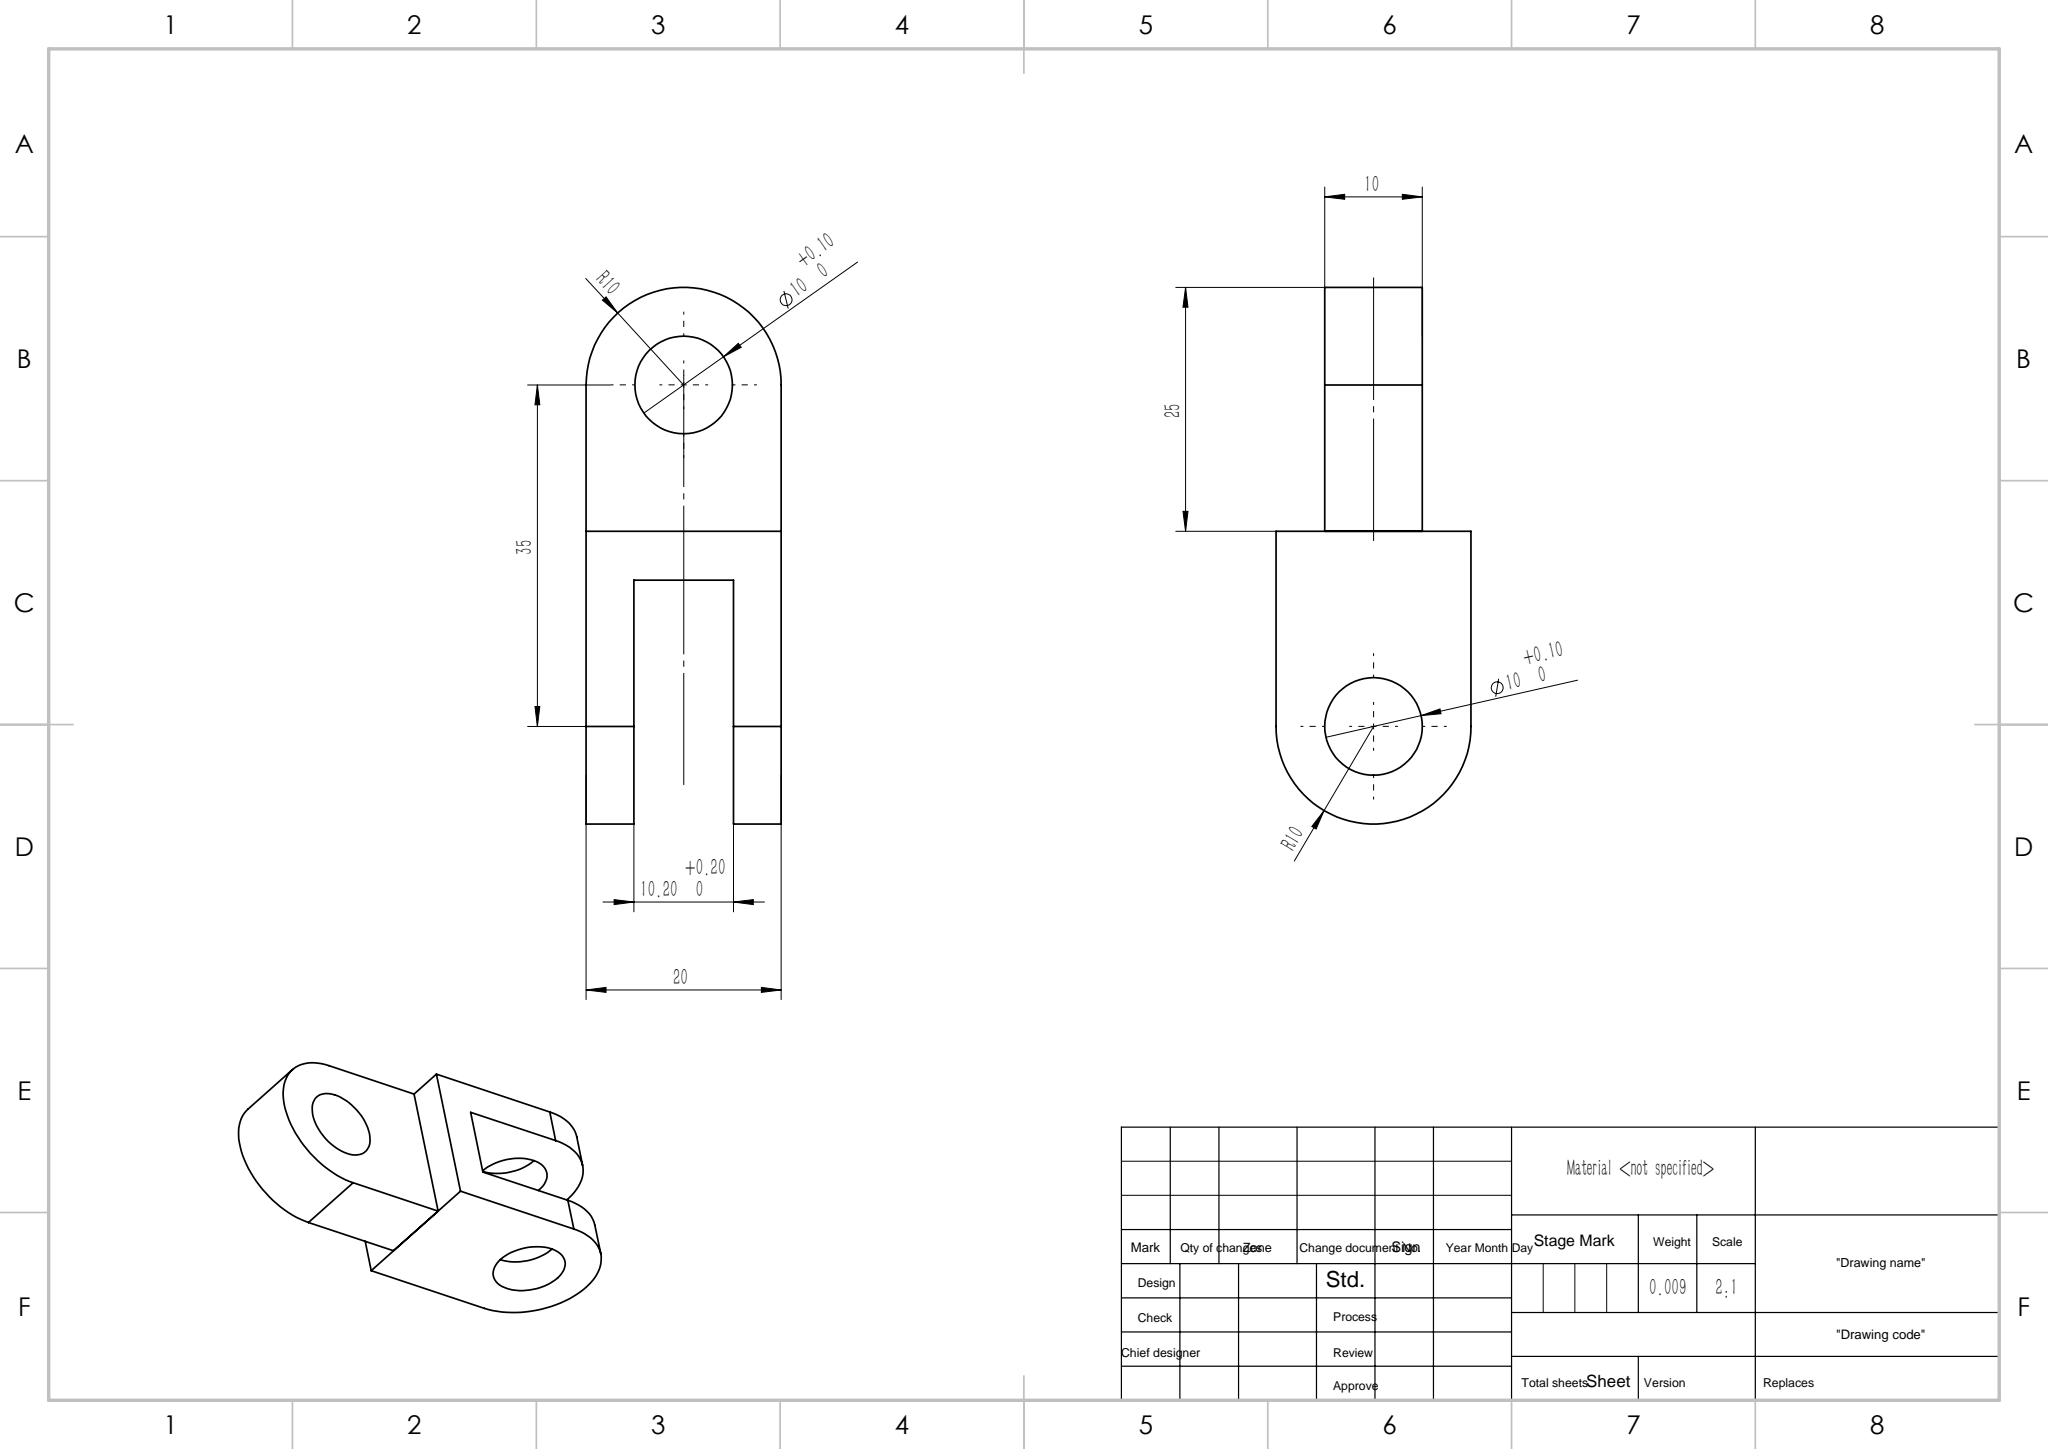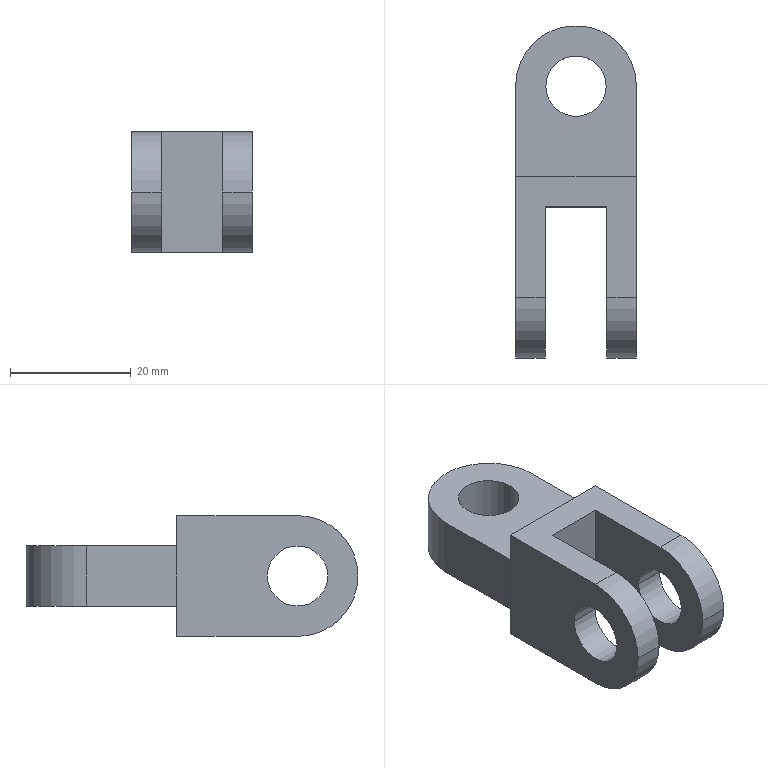Part | SolidWorks | features ICE 2, Extrusion 1 | 2 solids | 24 faces | box 20 x 55 x 20 mm | volume 9495 mm3 | plane 13 | cylinder 11 | commonest cylinder face diameters 10 x6 20 x5
STEP:
#1=CARTESIAN_POINT('',(-5.,0.,10.));
#2=VERTEX_POINT('',#1);
#3=CARTESIAN_POINT('',(5.,0.,10.));
#4=VERTEX_POINT('',#3);
#5=CARTESIAN_POINT('',(0.,0.,10.));
#6=DIRECTION('',(0.,0.,1.));
#7=DIRECTION('',(1.,0.,0.));
#8=AXIS2_PLACEMENT_3D('',#5,#6,#7);
#9=CIRCLE('',#8,5.);
#10=EDGE_CURVE('',#2,#4,#9,.T.);
#11=ORIENTED_EDGE('',*,*,#10,.T.);
#12=CARTESIAN_POINT('',(5.,0.,0.));
#13=VERTEX_POINT('',#12);
#14=CARTESIAN_POINT('',(5.,0.,10.));
#15=DIRECTION('',(0.,0.,-1.));
#16=VECTOR('',#15,1000.);
#17=LINE('',#14,#16);
#18=EDGE_CURVE('',#4,#13,#17,.T.);
#19=ORIENTED_EDGE('',*,*,#18,.T.);
#20=CARTESIAN_POINT('',(-5.,0.,0.));
#21=VERTEX_POINT('',#20);
#22=CARTESIAN_POINT('',(0.,0.,0.));
#23=DIRECTION('',(0.,0.,1.));
#24=DIRECTION('',(1.,0.,0.));
#25=AXIS2_PLACEMENT_3D('',#22,#23,#24);
#26=CIRCLE('',#25,5.);
#27=EDGE_CURVE('',#21,#13,#26,.T.);
#28=ORIENTED_EDGE('',*,*,#27,.F.);
#29=CARTESIAN_POINT('',(-5.,0.,10.));
#30=DIRECTION('',(0.,0.,-1.));
#31=VECTOR('',#30,1000.);
#32=LINE('',#29,#31);
#33=EDGE_CURVE('',#2,#21,#32,.T.);
#34=ORIENTED_EDGE('',*,*,#33,.F.);
#35=EDGE_LOOP('',(#11,#19,#28,#34));
#36=FACE_OUTER_BOUND('',#35,.T.);
#37=CARTESIAN_POINT('',(0.,0.,10.));
#38=DIRECTION('',(0.,0.,-1.));
#39=DIRECTION('',(-1.,0.,0.));
#40=AXIS2_PLACEMENT_3D('',#37,#38,#39);
#41=CYLINDRICAL_SURFACE('',#40,5.);
#42=ADVANCED_FACE('',(#36),#41,.F.);
#43=CARTESIAN_POINT('',(10.,0.,10.));
#44=VERTEX_POINT('',#43);
#45=CARTESIAN_POINT('',(-10.,0.,10.));
#46=VERTEX_POINT('',#45);
#47=CARTESIAN_POINT('',(0.,0.,10.));
#48=DIRECTION('',(0.,0.,1.));
#49=DIRECTION('',(1.,0.,0.));
#50=AXIS2_PLACEMENT_3D('',#47,#48,#49);
#51=CIRCLE('',#50,10.);
#52=EDGE_CURVE('',#44,#46,#51,.T.);
#53=ORIENTED_EDGE('',*,*,#52,.T.);
#54=CARTESIAN_POINT('',(-10.,-15.,10.));
#55=VERTEX_POINT('',#54);
#56=CARTESIAN_POINT('',(-10.,0.,10.));
#57=DIRECTION('',(0.,-1.,0.));
#58=VECTOR('',#57,1000.);
#59=LINE('',#56,#58);
#60=EDGE_CURVE('',#46,#55,#59,.T.);
#61=ORIENTED_EDGE('',*,*,#60,.T.);
#62=CARTESIAN_POINT('',(10.,-15.,10.));
#63=VERTEX_POINT('',#62);
#64=CARTESIAN_POINT('',(-10.,-15.,10.));
#65=DIRECTION('',(1.,0.,0.));
#66=VECTOR('',#65,1000.);
#67=LINE('',#64,#66);
#68=EDGE_CURVE('',#55,#63,#67,.T.);
#69=ORIENTED_EDGE('',*,*,#68,.T.);
#70=CARTESIAN_POINT('',(10.,-15.,10.));
#71=DIRECTION('',(0.,1.,0.));
#72=VECTOR('',#71,1000.);
#73=LINE('',#70,#72);
#74=EDGE_CURVE('',#63,#44,#73,.T.);
#75=ORIENTED_EDGE('',*,*,#74,.T.);
#76=EDGE_LOOP('',(#53,#61,#69,#75));
#77=FACE_OUTER_BOUND('',#76,.T.);
#78=ORIENTED_EDGE('',*,*,#10,.F.);
#79=CARTESIAN_POINT('',(0.,0.,10.));
#80=DIRECTION('',(0.,0.,1.));
#81=DIRECTION('',(1.,0.,0.));
#82=AXIS2_PLACEMENT_3D('',#79,#80,#81);
#83=CIRCLE('',#82,5.);
#84=EDGE_CURVE('',#4,#2,#83,.T.);
#85=ORIENTED_EDGE('',*,*,#84,.F.);
#86=EDGE_LOOP('',(#78,#85));
#87=FACE_BOUND('',#86,.T.);
#88=CARTESIAN_POINT('',(0.,0.,10.));
#89=DIRECTION('',(0.,0.,1.));
#90=DIRECTION('',(1.,0.,0.));
#91=AXIS2_PLACEMENT_3D('',#88,#89,#90);
#92=PLANE('',#91);
#93=ADVANCED_FACE('',(#77,#87),#92,.T.);
#94=CARTESIAN_POINT('',(10.,0.,0.));
#95=VERTEX_POINT('',#94);
#96=CARTESIAN_POINT('',(-10.,0.,0.));
#97=VERTEX_POINT('',#96);
#98=CARTESIAN_POINT('',(0.,0.,0.));
#99=DIRECTION('',(0.,0.,1.));
#100=DIRECTION('',(1.,0.,0.));
#101=AXIS2_PLACEMENT_3D('',#98,#99,#100);
#102=CIRCLE('',#101,10.);
#103=EDGE_CURVE('',#95,#97,#102,.T.);
#104=ORIENTED_EDGE('',*,*,#103,.F.);
#105=CARTESIAN_POINT('',(10.,-15.,0.));
#106=VERTEX_POINT('',#105);
#107=CARTESIAN_POINT('',(10.,-15.,0.));
#108=DIRECTION('',(0.,1.,0.));
#109=VECTOR('',#108,1000.);
#110=LINE('',#107,#109);
#111=EDGE_CURVE('',#106,#95,#110,.T.);
#112=ORIENTED_EDGE('',*,*,#111,.F.);
#113=CARTESIAN_POINT('',(-10.,-15.,0.));
#114=VERTEX_POINT('',#113);
#115=CARTESIAN_POINT('',(-10.,-15.,0.));
#116=DIRECTION('',(1.,0.,0.));
#117=VECTOR('',#116,1000.);
#118=LINE('',#115,#117);
#119=EDGE_CURVE('',#114,#106,#118,.T.);
#120=ORIENTED_EDGE('',*,*,#119,.F.);
#121=CARTESIAN_POINT('',(-10.,0.,0.));
#122=DIRECTION('',(0.,-1.,0.));
#123=VECTOR('',#122,1000.);
#124=LINE('',#121,#123);
#125=EDGE_CURVE('',#97,#114,#124,.T.);
#126=ORIENTED_EDGE('',*,*,#125,.F.);
#127=EDGE_LOOP('',(#104,#112,#120,#126));
#128=FACE_OUTER_BOUND('',#127,.T.);
#129=ORIENTED_EDGE('',*,*,#27,.T.);
#130=CARTESIAN_POINT('',(0.,0.,0.));
#131=DIRECTION('',(0.,0.,1.));
#132=DIRECTION('',(1.,0.,0.));
#133=AXIS2_PLACEMENT_3D('',#130,#131,#132);
#134=CIRCLE('',#133,5.);
#135=EDGE_CURVE('',#13,#21,#134,.T.);
#136=ORIENTED_EDGE('',*,*,#135,.T.);
#137=EDGE_LOOP('',(#129,#136));
#138=FACE_BOUND('',#137,.T.);
#139=CARTESIAN_POINT('',(0.,0.,0.));
#140=DIRECTION('',(0.,0.,1.));
#141=DIRECTION('',(1.,0.,0.));
#142=AXIS2_PLACEMENT_3D('',#139,#140,#141);
#143=PLANE('',#142);
#144=ADVANCED_FACE('',(#128,#138),#143,.F.);
#145=ORIENTED_EDGE('',*,*,#103,.T.);
#146=CARTESIAN_POINT('',(-10.,0.,10.));
#147=DIRECTION('',(0.,0.,-1.));
#148=VECTOR('',#147,1000.);
#149=LINE('',#146,#148);
#150=EDGE_CURVE('',#46,#97,#149,.T.);
#151=ORIENTED_EDGE('',*,*,#150,.F.);
#152=ORIENTED_EDGE('',*,*,#52,.F.);
#153=CARTESIAN_POINT('',(10.,0.,10.));
#154=DIRECTION('',(0.,0.,-1.));
#155=VECTOR('',#154,1000.);
#156=LINE('',#153,#155);
#157=EDGE_CURVE('',#44,#95,#156,.T.);
#158=ORIENTED_EDGE('',*,*,#157,.T.);
#159=EDGE_LOOP('',(#145,#151,#152,#158));
#160=FACE_OUTER_BOUND('',#159,.T.);
#161=CARTESIAN_POINT('',(0.,0.,10.));
#162=DIRECTION('',(0.,0.,-1.));
#163=DIRECTION('',(-1.,0.,0.));
#164=AXIS2_PLACEMENT_3D('',#161,#162,#163);
#165=CYLINDRICAL_SURFACE('',#164,10.);
#166=ADVANCED_FACE('',(#160),#165,.T.);
#167=ORIENTED_EDGE('',*,*,#125,.T.);
#168=CARTESIAN_POINT('',(-10.,-15.,10.));
#169=DIRECTION('',(0.,0.,-1.));
#170=VECTOR('',#169,1000.);
#171=LINE('',#168,#170);
#172=EDGE_CURVE('',#55,#114,#171,.T.);
#173=ORIENTED_EDGE('',*,*,#172,.F.);
#174=ORIENTED_EDGE('',*,*,#60,.F.);
#175=ORIENTED_EDGE('',*,*,#150,.T.);
#176=EDGE_LOOP('',(#167,#173,#174,#175));
#177=FACE_OUTER_BOUND('',#176,.T.);
#178=CARTESIAN_POINT('',(-10.,0.,10.));
#179=DIRECTION('',(1.,0.,0.));
#180=DIRECTION('',(0.,1.,0.));
#181=AXIS2_PLACEMENT_3D('',#178,#179,#180);
#182=PLANE('',#181);
#183=ADVANCED_FACE('',(#177),#182,.F.);
#184=ORIENTED_EDGE('',*,*,#119,.T.);
#185=CARTESIAN_POINT('',(10.,-15.,10.));
#186=DIRECTION('',(0.,0.,-1.));
#187=VECTOR('',#186,1000.);
#188=LINE('',#185,#187);
#189=EDGE_CURVE('',#63,#106,#188,.T.);
#190=ORIENTED_EDGE('',*,*,#189,.F.);
#191=ORIENTED_EDGE('',*,*,#68,.F.);
#192=ORIENTED_EDGE('',*,*,#172,.T.);
#193=EDGE_LOOP('',(#184,#190,#191,#192));
#194=FACE_OUTER_BOUND('',#193,.T.);
#195=CARTESIAN_POINT('',(-10.,-15.,10.));
#196=DIRECTION('',(0.,1.,0.));
#197=DIRECTION('',(0.,0.,1.));
#198=AXIS2_PLACEMENT_3D('',#195,#196,#197);
#199=PLANE('',#198);
#200=ADVANCED_FACE('',(#194),#199,.F.);
#201=ORIENTED_EDGE('',*,*,#111,.T.);
#202=ORIENTED_EDGE('',*,*,#157,.F.);
#203=ORIENTED_EDGE('',*,*,#74,.F.);
#204=ORIENTED_EDGE('',*,*,#189,.T.);
#205=EDGE_LOOP('',(#201,#202,#203,#204));
#206=FACE_OUTER_BOUND('',#205,.T.);
#207=CARTESIAN_POINT('',(10.,-15.,10.));
#208=DIRECTION('',(-1.,0.,0.));
#209=DIRECTION('',(0.,-1.,0.));
#210=AXIS2_PLACEMENT_3D('',#207,#208,#209);
#211=PLANE('',#210);
#212=ADVANCED_FACE('',(#206),#211,.F.);
#213=ORIENTED_EDGE('',*,*,#18,.F.);
#214=ORIENTED_EDGE('',*,*,#84,.T.);
#215=ORIENTED_EDGE('',*,*,#33,.T.);
#216=ORIENTED_EDGE('',*,*,#135,.F.);
#217=EDGE_LOOP('',(#213,#214,#215,#216));
#218=FACE_OUTER_BOUND('',#217,.T.);
#219=CARTESIAN_POINT('',(0.,0.,10.));
#220=DIRECTION('',(0.,0.,-1.));
#221=DIRECTION('',(-1.,0.,0.));
#222=AXIS2_PLACEMENT_3D('',#219,#220,#221);
#223=CYLINDRICAL_SURFACE('',#222,5.);
#224=ADVANCED_FACE('',(#218),#223,.F.);
#225=CLOSED_SHELL('',(#42,#93,#144,#166,#183,#200,#212,#224));
#226=MANIFOLD_SOLID_BREP('',#225);
#227=CARTESIAN_POINT('',(10.,-30.,5.));
#228=VERTEX_POINT('',#227);
#229=CARTESIAN_POINT('',(10.,-40.,5.));
#230=VERTEX_POINT('',#229);
#231=CARTESIAN_POINT('',(10.,-35.,5.));
#232=DIRECTION('',(-1.,0.,0.));
#233=DIRECTION('',(0.,-1.,0.));
#234=AXIS2_PLACEMENT_3D('',#231,#232,#233);
#235=CIRCLE('',#234,5.);
#236=EDGE_CURVE('',#228,#230,#235,.T.);
#237=ORIENTED_EDGE('',*,*,#236,.F.);
#238=CARTESIAN_POINT('',(5.1,-30.,5.));
#239=VERTEX_POINT('',#238);
#240=CARTESIAN_POINT('',(10.,-30.,5.));
#241=DIRECTION('',(-1.,0.,0.));
#242=VECTOR('',#241,1000.);
#243=LINE('',#240,#242);
#244=EDGE_CURVE('',#228,#239,#243,.T.);
#245=ORIENTED_EDGE('',*,*,#244,.T.);
#246=CARTESIAN_POINT('',(5.1,-40.,5.));
#247=VERTEX_POINT('',#246);
#248=CARTESIAN_POINT('',(5.1,-35.,5.));
#249=DIRECTION('',(-1.,0.,0.));
#250=DIRECTION('',(0.,1.,0.));
#251=AXIS2_PLACEMENT_3D('',#248,#249,#250);
#252=CIRCLE('',#251,5.);
#253=EDGE_CURVE('',#239,#247,#252,.T.);
#254=ORIENTED_EDGE('',*,*,#253,.T.);
#255=CARTESIAN_POINT('',(10.,-40.,5.));
#256=DIRECTION('',(-1.,0.,0.));
#257=VECTOR('',#256,1000.);
#258=LINE('',#255,#257);
#259=EDGE_CURVE('',#230,#247,#258,.T.);
#260=ORIENTED_EDGE('',*,*,#259,.F.);
#261=EDGE_LOOP('',(#237,#245,#254,#260));
#262=FACE_OUTER_BOUND('',#261,.T.);
#263=CARTESIAN_POINT('',(10.,-35.,5.));
#264=DIRECTION('',(-1.,0.,0.));
#265=DIRECTION('',(0.,-1.,0.));
#266=AXIS2_PLACEMENT_3D('',#263,#264,#265);
#267=CYLINDRICAL_SURFACE('',#266,5.);
#268=ADVANCED_FACE('',(#262),#267,.F.);
#269=CARTESIAN_POINT('',(10.,-35.,-5.));
#270=VERTEX_POINT('',#269);
#271=CARTESIAN_POINT('',(10.,-45.,5.));
#272=VERTEX_POINT('',#271);
#273=CARTESIAN_POINT('',(10.,-35.,5.));
#274=DIRECTION('',(-1.,0.,0.));
#275=DIRECTION('',(0.,-1.,0.));
#276=AXIS2_PLACEMENT_3D('',#273,#274,#275);
#277=CIRCLE('',#276,10.);
#278=EDGE_CURVE('',#270,#272,#277,.T.);
#279=ORIENTED_EDGE('',*,*,#278,.T.);
#280=CARTESIAN_POINT('',(5.1,-45.,5.));
#281=VERTEX_POINT('',#280);
#282=CARTESIAN_POINT('',(10.,-45.,5.));
#283=DIRECTION('',(-1.,0.,0.));
#284=VECTOR('',#283,1000.);
#285=LINE('',#282,#284);
#286=EDGE_CURVE('',#272,#281,#285,.T.);
#287=ORIENTED_EDGE('',*,*,#286,.T.);
#288=CARTESIAN_POINT('',(5.1,-35.,-5.));
#289=VERTEX_POINT('',#288);
#290=CARTESIAN_POINT('',(5.1,-35.,5.));
#291=DIRECTION('',(-1.,0.,0.));
#292=DIRECTION('',(0.,1.,0.));
#293=AXIS2_PLACEMENT_3D('',#290,#291,#292);
#294=CIRCLE('',#293,10.);
#295=EDGE_CURVE('',#289,#281,#294,.T.);
#296=ORIENTED_EDGE('',*,*,#295,.F.);
#297=CARTESIAN_POINT('',(10.,-35.,-5.));
#298=DIRECTION('',(-1.,0.,0.));
#299=VECTOR('',#298,1000.);
#300=LINE('',#297,#299);
#301=EDGE_CURVE('',#270,#289,#300,.T.);
#302=ORIENTED_EDGE('',*,*,#301,.F.);
#303=EDGE_LOOP('',(#279,#287,#296,#302));
#304=FACE_OUTER_BOUND('',#303,.T.);
#305=CARTESIAN_POINT('',(10.,-35.,5.));
#306=DIRECTION('',(-1.,0.,0.));
#307=DIRECTION('',(0.,-1.,0.));
#308=AXIS2_PLACEMENT_3D('',#305,#306,#307);
#309=CYLINDRICAL_SURFACE('',#308,10.);
#310=ADVANCED_FACE('',(#304),#309,.T.);
#311=CARTESIAN_POINT('',(-5.1,-40.,5.));
#312=VERTEX_POINT('',#311);
#313=CARTESIAN_POINT('',(-5.1,-30.,5.));
#314=VERTEX_POINT('',#313);
#315=CARTESIAN_POINT('',(-5.1,-35.,5.));
#316=DIRECTION('',(1.,0.,0.));
#317=DIRECTION('',(0.,-1.,0.));
#318=AXIS2_PLACEMENT_3D('',#315,#316,#317);
#319=CIRCLE('',#318,5.);
#320=EDGE_CURVE('',#312,#314,#319,.T.);
#321=ORIENTED_EDGE('',*,*,#320,.T.);
#322=CARTESIAN_POINT('',(-10.,-30.,5.));
#323=VERTEX_POINT('',#322);
#324=CARTESIAN_POINT('',(10.,-30.,5.));
#325=DIRECTION('',(-1.,0.,0.));
#326=VECTOR('',#325,1000.);
#327=LINE('',#324,#326);
#328=EDGE_CURVE('',#314,#323,#327,.T.);
#329=ORIENTED_EDGE('',*,*,#328,.T.);
#330=CARTESIAN_POINT('',(-10.,-40.,5.));
#331=VERTEX_POINT('',#330);
#332=CARTESIAN_POINT('',(-10.,-35.,5.));
#333=DIRECTION('',(-1.,0.,0.));
#334=DIRECTION('',(0.,-1.,0.));
#335=AXIS2_PLACEMENT_3D('',#332,#333,#334);
#336=CIRCLE('',#335,5.);
#337=EDGE_CURVE('',#323,#331,#336,.T.);
#338=ORIENTED_EDGE('',*,*,#337,.T.);
#339=CARTESIAN_POINT('',(10.,-40.,5.));
#340=DIRECTION('',(-1.,0.,0.));
#341=VECTOR('',#340,1000.);
#342=LINE('',#339,#341);
#343=EDGE_CURVE('',#312,#331,#342,.T.);
#344=ORIENTED_EDGE('',*,*,#343,.F.);
#345=EDGE_LOOP('',(#321,#329,#338,#344));
#346=FACE_OUTER_BOUND('',#345,.T.);
#347=CARTESIAN_POINT('',(10.,-35.,5.));
#348=DIRECTION('',(-1.,0.,0.));
#349=DIRECTION('',(0.,-1.,0.));
#350=AXIS2_PLACEMENT_3D('',#347,#348,#349);
#351=CYLINDRICAL_SURFACE('',#350,5.);
#352=ADVANCED_FACE('',(#346),#351,.F.);
#353=CARTESIAN_POINT('',(-5.1,-45.,5.));
#354=VERTEX_POINT('',#353);
#355=CARTESIAN_POINT('',(-5.1,-35.,-5.));
#356=VERTEX_POINT('',#355);
#357=CARTESIAN_POINT('',(-5.1,-35.,5.));
#358=DIRECTION('',(1.,0.,0.));
#359=DIRECTION('',(0.,-1.,0.));
#360=AXIS2_PLACEMENT_3D('',#357,#358,#359);
#361=CIRCLE('',#360,10.);
#362=EDGE_CURVE('',#354,#356,#361,.T.);
#363=ORIENTED_EDGE('',*,*,#362,.F.);
#364=CARTESIAN_POINT('',(-10.,-45.,5.));
#365=VERTEX_POINT('',#364);
#366=CARTESIAN_POINT('',(10.,-45.,5.));
#367=DIRECTION('',(-1.,0.,0.));
#368=VECTOR('',#367,1000.);
#369=LINE('',#366,#368);
#370=EDGE_CURVE('',#354,#365,#369,.T.);
#371=ORIENTED_EDGE('',*,*,#370,.T.);
#372=CARTESIAN_POINT('',(-10.,-35.,-5.));
#373=VERTEX_POINT('',#372);
#374=CARTESIAN_POINT('',(-10.,-35.,5.));
#375=DIRECTION('',(-1.,0.,0.));
#376=DIRECTION('',(0.,-1.,0.));
#377=AXIS2_PLACEMENT_3D('',#374,#375,#376);
#378=CIRCLE('',#377,10.);
#379=EDGE_CURVE('',#373,#365,#378,.T.);
#380=ORIENTED_EDGE('',*,*,#379,.F.);
#381=CARTESIAN_POINT('',(10.,-35.,-5.));
#382=DIRECTION('',(-1.,0.,0.));
#383=VECTOR('',#382,1000.);
#384=LINE('',#381,#383);
#385=EDGE_CURVE('',#356,#373,#384,.T.);
#386=ORIENTED_EDGE('',*,*,#385,.F.);
#387=EDGE_LOOP('',(#363,#371,#380,#386));
#388=FACE_OUTER_BOUND('',#387,.T.);
#389=CARTESIAN_POINT('',(10.,-35.,5.));
#390=DIRECTION('',(-1.,0.,0.));
#391=DIRECTION('',(0.,-1.,0.));
#392=AXIS2_PLACEMENT_3D('',#389,#390,#391);
#393=CYLINDRICAL_SURFACE('',#392,10.);
#394=ADVANCED_FACE('',(#388),#393,.T.);
#395=ORIENTED_EDGE('',*,*,#370,.F.);
#396=CARTESIAN_POINT('',(-5.1,-35.,15.));
#397=VERTEX_POINT('',#396);
#398=CARTESIAN_POINT('',(-5.1,-35.,5.));
#399=DIRECTION('',(1.,0.,0.));
#400=DIRECTION('',(0.,-1.,0.));
#401=AXIS2_PLACEMENT_3D('',#398,#399,#400);
#402=CIRCLE('',#401,10.);
#403=EDGE_CURVE('',#397,#354,#402,.T.);
#404=ORIENTED_EDGE('',*,*,#403,.F.);
#405=CARTESIAN_POINT('',(-10.,-35.,15.));
#406=VERTEX_POINT('',#405);
#407=CARTESIAN_POINT('',(10.,-35.,15.));
#408=DIRECTION('',(-1.,0.,0.));
#409=VECTOR('',#408,1000.);
#410=LINE('',#407,#409);
#411=EDGE_CURVE('',#397,#406,#410,.T.);
#412=ORIENTED_EDGE('',*,*,#411,.T.);
#413=CARTESIAN_POINT('',(-10.,-35.,5.));
#414=DIRECTION('',(-1.,0.,0.));
#415=DIRECTION('',(0.,-1.,0.));
#416=AXIS2_PLACEMENT_3D('',#413,#414,#415);
#417=CIRCLE('',#416,10.);
#418=EDGE_CURVE('',#365,#406,#417,.T.);
#419=ORIENTED_EDGE('',*,*,#418,.F.);
#420=EDGE_LOOP('',(#395,#404,#412,#419));
#421=FACE_OUTER_BOUND('',#420,.T.);
#422=CARTESIAN_POINT('',(10.,-35.,5.));
#423=DIRECTION('',(-1.,0.,0.));
#424=DIRECTION('',(0.,-1.,0.));
#425=AXIS2_PLACEMENT_3D('',#422,#423,#424);
#426=CYLINDRICAL_SURFACE('',#425,10.);
#427=ADVANCED_FACE('',(#421),#426,.T.);
#428=ORIENTED_EDGE('',*,*,#328,.F.);
#429=CARTESIAN_POINT('',(-5.1,-35.,5.));
#430=DIRECTION('',(1.,0.,0.));
#431=DIRECTION('',(0.,-1.,0.));
#432=AXIS2_PLACEMENT_3D('',#429,#430,#431);
#433=CIRCLE('',#432,5.);
#434=EDGE_CURVE('',#314,#312,#433,.T.);
#435=ORIENTED_EDGE('',*,*,#434,.T.);
#436=ORIENTED_EDGE('',*,*,#343,.T.);
#437=CARTESIAN_POINT('',(-10.,-35.,5.));
#438=DIRECTION('',(-1.,0.,0.));
#439=DIRECTION('',(0.,-1.,0.));
#440=AXIS2_PLACEMENT_3D('',#437,#438,#439);
#441=CIRCLE('',#440,5.);
#442=EDGE_CURVE('',#331,#323,#441,.T.);
#443=ORIENTED_EDGE('',*,*,#442,.T.);
#444=EDGE_LOOP('',(#428,#435,#436,#443));
#445=FACE_OUTER_BOUND('',#444,.T.);
#446=CARTESIAN_POINT('',(10.,-35.,5.));
#447=DIRECTION('',(-1.,0.,0.));
#448=DIRECTION('',(0.,-1.,0.));
#449=AXIS2_PLACEMENT_3D('',#446,#447,#448);
#450=CYLINDRICAL_SURFACE('',#449,5.);
#451=ADVANCED_FACE('',(#445),#450,.F.);
#452=ORIENTED_EDGE('',*,*,#286,.F.);
#453=CARTESIAN_POINT('',(10.,-35.,15.));
#454=VERTEX_POINT('',#453);
#455=CARTESIAN_POINT('',(10.,-35.,5.));
#456=DIRECTION('',(-1.,0.,0.));
#457=DIRECTION('',(0.,-1.,0.));
#458=AXIS2_PLACEMENT_3D('',#455,#456,#457);
#459=CIRCLE('',#458,10.);
#460=EDGE_CURVE('',#272,#454,#459,.T.);
#461=ORIENTED_EDGE('',*,*,#460,.T.);
#462=CARTESIAN_POINT('',(5.1,-35.,15.));
#463=VERTEX_POINT('',#462);
#464=CARTESIAN_POINT('',(10.,-35.,15.));
#465=DIRECTION('',(-1.,0.,0.));
#466=VECTOR('',#465,1000.);
#467=LINE('',#464,#466);
#468=EDGE_CURVE('',#454,#463,#467,.T.);
#469=ORIENTED_EDGE('',*,*,#468,.T.);
#470=CARTESIAN_POINT('',(5.1,-35.,5.));
#471=DIRECTION('',(-1.,0.,0.));
#472=DIRECTION('',(0.,1.,0.));
#473=AXIS2_PLACEMENT_3D('',#470,#471,#472);
#474=CIRCLE('',#473,10.);
#475=EDGE_CURVE('',#281,#463,#474,.T.);
#476=ORIENTED_EDGE('',*,*,#475,.F.);
#477=EDGE_LOOP('',(#452,#461,#469,#476));
#478=FACE_OUTER_BOUND('',#477,.T.);
#479=CARTESIAN_POINT('',(10.,-35.,5.));
#480=DIRECTION('',(-1.,0.,0.));
#481=DIRECTION('',(0.,-1.,0.));
#482=AXIS2_PLACEMENT_3D('',#479,#480,#481);
#483=CYLINDRICAL_SURFACE('',#482,10.);
#484=ADVANCED_FACE('',(#478),#483,.T.);
#485=CARTESIAN_POINT('',(-5.1,-20.,-5.));
#486=VERTEX_POINT('',#485);
#487=CARTESIAN_POINT('',(-5.1,-20.,-5.));
#488=DIRECTION('',(0.,1.,0.));
#489=VECTOR('',#488,1000.);
#490=LINE('',#487,#489);
#491=EDGE_CURVE('',#356,#486,#490,.T.);
#492=ORIENTED_EDGE('',*,*,#491,.F.);
#493=ORIENTED_EDGE('',*,*,#385,.T.);
#494=CARTESIAN_POINT('',(-10.,-15.,-5.));
#495=VERTEX_POINT('',#494);
#496=CARTESIAN_POINT('',(-10.,-15.,-5.));
#497=DIRECTION('',(0.,-1.,0.));
#498=VECTOR('',#497,1000.);
#499=LINE('',#496,#498);
#500=EDGE_CURVE('',#495,#373,#499,.T.);
#501=ORIENTED_EDGE('',*,*,#500,.F.);
#502=CARTESIAN_POINT('',(10.,-15.,-5.));
#503=VERTEX_POINT('',#502);
#504=CARTESIAN_POINT('',(10.,-15.,-5.));
#505=DIRECTION('',(-1.,0.,0.));
#506=VECTOR('',#505,1000.);
#507=LINE('',#504,#506);
#508=EDGE_CURVE('',#503,#495,#507,.T.);
#509=ORIENTED_EDGE('',*,*,#508,.F.);
#510=CARTESIAN_POINT('',(10.,-15.,-5.));
#511=DIRECTION('',(0.,-1.,0.));
#512=VECTOR('',#511,1000.);
#513=LINE('',#510,#512);
#514=EDGE_CURVE('',#503,#270,#513,.T.);
#515=ORIENTED_EDGE('',*,*,#514,.T.);
#516=ORIENTED_EDGE('',*,*,#301,.T.);
#517=CARTESIAN_POINT('',(5.1,-20.,-5.));
#518=VERTEX_POINT('',#517);
#519=CARTESIAN_POINT('',(5.1,-20.,-5.));
#520=DIRECTION('',(0.,-1.,0.));
#521=VECTOR('',#520,1000.);
#522=LINE('',#519,#521);
#523=EDGE_CURVE('',#518,#289,#522,.T.);
#524=ORIENTED_EDGE('',*,*,#523,.F.);
#525=CARTESIAN_POINT('',(-5.1,-20.,-5.));
#526=DIRECTION('',(1.,0.,0.));
#527=VECTOR('',#526,1000.);
#528=LINE('',#525,#527);
#529=EDGE_CURVE('',#486,#518,#528,.T.);
#530=ORIENTED_EDGE('',*,*,#529,.F.);
#531=EDGE_LOOP('',(#492,#493,#501,#509,#515,#516,#524,#530));
#532=FACE_OUTER_BOUND('',#531,.T.);
#533=CARTESIAN_POINT('',(10.,-15.,-5.));
#534=DIRECTION('',(0.,0.,-1.));
#535=DIRECTION('',(-1.,0.,0.));
#536=AXIS2_PLACEMENT_3D('',#533,#534,#535);
#537=PLANE('',#536);
#538=ADVANCED_FACE('',(#532),#537,.T.);
#539=CARTESIAN_POINT('',(-10.,-15.,15.));
#540=VERTEX_POINT('',#539);
#541=CARTESIAN_POINT('',(-10.,-15.,15.));
#542=DIRECTION('',(0.,0.,-1.));
#543=VECTOR('',#542,1000.);
#544=LINE('',#541,#543);
#545=EDGE_CURVE('',#540,#495,#544,.T.);
#546=ORIENTED_EDGE('',*,*,#545,.F.);
#547=CARTESIAN_POINT('',(10.,-15.,15.));
#548=VERTEX_POINT('',#547);
#549=CARTESIAN_POINT('',(10.,-15.,15.));
#550=DIRECTION('',(-1.,0.,0.));
#551=VECTOR('',#550,1000.);
#552=LINE('',#549,#551);
#553=EDGE_CURVE('',#548,#540,#552,.T.);
#554=ORIENTED_EDGE('',*,*,#553,.F.);
#555=CARTESIAN_POINT('',(10.,-15.,15.));
#556=DIRECTION('',(0.,0.,-1.));
#557=VECTOR('',#556,1000.);
#558=LINE('',#555,#557);
#559=EDGE_CURVE('',#548,#503,#558,.T.);
#560=ORIENTED_EDGE('',*,*,#559,.T.);
#561=ORIENTED_EDGE('',*,*,#508,.T.);
#562=EDGE_LOOP('',(#546,#554,#560,#561));
#563=FACE_OUTER_BOUND('',#562,.T.);
#564=CARTESIAN_POINT('',(10.,-15.,15.));
#565=DIRECTION('',(0.,1.,0.));
#566=DIRECTION('',(-1.,0.,0.));
#567=AXIS2_PLACEMENT_3D('',#564,#565,#566);
#568=PLANE('',#567);
#569=ADVANCED_FACE('',(#563),#568,.T.);
#570=CARTESIAN_POINT('',(-5.1,-20.,15.));
#571=VERTEX_POINT('',#570);
#572=CARTESIAN_POINT('',(-5.1,-20.,15.));
#573=DIRECTION('',(0.,1.,0.));
#574=VECTOR('',#573,1000.);
#575=LINE('',#572,#574);
#576=EDGE_CURVE('',#397,#571,#575,.T.);
#577=ORIENTED_EDGE('',*,*,#576,.T.);
#578=CARTESIAN_POINT('',(5.1,-20.,15.));
#579=VERTEX_POINT('',#578);
#580=CARTESIAN_POINT('',(-5.1,-20.,15.));
#581=DIRECTION('',(1.,0.,0.));
#582=VECTOR('',#581,1000.);
#583=LINE('',#580,#582);
#584=EDGE_CURVE('',#571,#579,#583,.T.);
#585=ORIENTED_EDGE('',*,*,#584,.T.);
#586=CARTESIAN_POINT('',(5.1,-20.,15.));
#587=DIRECTION('',(0.,-1.,0.));
#588=VECTOR('',#587,1000.);
#589=LINE('',#586,#588);
#590=EDGE_CURVE('',#579,#463,#589,.T.);
#591=ORIENTED_EDGE('',*,*,#590,.T.);
#592=ORIENTED_EDGE('',*,*,#468,.F.);
#593=CARTESIAN_POINT('',(10.,-35.,15.));
#594=DIRECTION('',(0.,1.,0.));
#595=VECTOR('',#594,1000.);
#596=LINE('',#593,#595);
#597=EDGE_CURVE('',#454,#548,#596,.T.);
#598=ORIENTED_EDGE('',*,*,#597,.T.);
#599=ORIENTED_EDGE('',*,*,#553,.T.);
#600=CARTESIAN_POINT('',(-10.,-35.,15.));
#601=DIRECTION('',(0.,1.,0.));
#602=VECTOR('',#601,1000.);
#603=LINE('',#600,#602);
#604=EDGE_CURVE('',#406,#540,#603,.T.);
#605=ORIENTED_EDGE('',*,*,#604,.F.);
#606=ORIENTED_EDGE('',*,*,#411,.F.);
#607=EDGE_LOOP('',(#577,#585,#591,#592,#598,#599,#605,#606));
#608=FACE_OUTER_BOUND('',#607,.T.);
#609=CARTESIAN_POINT('',(10.,-35.,15.));
#610=DIRECTION('',(0.,0.,1.));
#611=DIRECTION('',(1.,0.,0.));
#612=AXIS2_PLACEMENT_3D('',#609,#610,#611);
#613=PLANE('',#612);
#614=ADVANCED_FACE('',(#608),#613,.T.);
#615=CARTESIAN_POINT('',(10.,-35.,5.));
#616=DIRECTION('',(-1.,0.,0.));
#617=DIRECTION('',(0.,-1.,0.));
#618=AXIS2_PLACEMENT_3D('',#615,#616,#617);
#619=CIRCLE('',#618,5.);
#620=EDGE_CURVE('',#230,#228,#619,.T.);
#621=ORIENTED_EDGE('',*,*,#620,.T.);
#622=ORIENTED_EDGE('',*,*,#236,.T.);
#623=EDGE_LOOP('',(#621,#622));
#624=FACE_BOUND('',#623,.T.);
#625=ORIENTED_EDGE('',*,*,#278,.F.);
#626=ORIENTED_EDGE('',*,*,#514,.F.);
#627=ORIENTED_EDGE('',*,*,#559,.F.);
#628=ORIENTED_EDGE('',*,*,#597,.F.);
#629=ORIENTED_EDGE('',*,*,#460,.F.);
#630=EDGE_LOOP('',(#625,#626,#627,#628,#629));
#631=FACE_OUTER_BOUND('',#630,.T.);
#632=CARTESIAN_POINT('',(10.,-35.,5.));
#633=DIRECTION('',(-1.,0.,0.));
#634=DIRECTION('',(0.,-1.,0.));
#635=AXIS2_PLACEMENT_3D('',#632,#633,#634);
#636=PLANE('',#635);
#637=ADVANCED_FACE('',(#624,#631),#636,.F.);
#638=ORIENTED_EDGE('',*,*,#442,.F.);
#639=ORIENTED_EDGE('',*,*,#337,.F.);
#640=EDGE_LOOP('',(#638,#639));
#641=FACE_BOUND('',#640,.T.);
#642=ORIENTED_EDGE('',*,*,#379,.T.);
#643=ORIENTED_EDGE('',*,*,#418,.T.);
#644=ORIENTED_EDGE('',*,*,#604,.T.);
#645=ORIENTED_EDGE('',*,*,#545,.T.);
#646=ORIENTED_EDGE('',*,*,#500,.T.);
#647=EDGE_LOOP('',(#642,#643,#644,#645,#646));
#648=FACE_OUTER_BOUND('',#647,.T.);
#649=CARTESIAN_POINT('',(-10.,-35.,5.));
#650=DIRECTION('',(-1.,0.,0.));
#651=DIRECTION('',(0.,-1.,0.));
#652=AXIS2_PLACEMENT_3D('',#649,#650,#651);
#653=PLANE('',#652);
#654=ADVANCED_FACE('',(#641,#648),#653,.T.);
#655=ORIENTED_EDGE('',*,*,#244,.F.);
#656=ORIENTED_EDGE('',*,*,#620,.F.);
#657=ORIENTED_EDGE('',*,*,#259,.T.);
#658=CARTESIAN_POINT('',(5.1,-35.,5.));
#659=DIRECTION('',(-1.,0.,0.));
#660=DIRECTION('',(0.,1.,0.));
#661=AXIS2_PLACEMENT_3D('',#658,#659,#660);
#662=CIRCLE('',#661,5.);
#663=EDGE_CURVE('',#247,#239,#662,.T.);
#664=ORIENTED_EDGE('',*,*,#663,.T.);
#665=EDGE_LOOP('',(#655,#656,#657,#664));
#666=FACE_OUTER_BOUND('',#665,.T.);
#667=CARTESIAN_POINT('',(10.,-35.,5.));
#668=DIRECTION('',(-1.,0.,0.));
#669=DIRECTION('',(0.,-1.,0.));
#670=AXIS2_PLACEMENT_3D('',#667,#668,#669);
#671=CYLINDRICAL_SURFACE('',#670,5.);
#672=ADVANCED_FACE('',(#666),#671,.F.);
#673=ORIENTED_EDGE('',*,*,#403,.T.);
#674=ORIENTED_EDGE('',*,*,#362,.T.);
#675=ORIENTED_EDGE('',*,*,#491,.T.);
#676=CARTESIAN_POINT('',(-5.1,-20.,15.));
#677=DIRECTION('',(0.,0.,-1.));
#678=VECTOR('',#677,1000.);
#679=LINE('',#676,#678);
#680=EDGE_CURVE('',#571,#486,#679,.T.);
#681=ORIENTED_EDGE('',*,*,#680,.F.);
#682=ORIENTED_EDGE('',*,*,#576,.F.);
#683=EDGE_LOOP('',(#673,#674,#675,#681,#682));
#684=FACE_OUTER_BOUND('',#683,.T.);
#685=ORIENTED_EDGE('',*,*,#320,.F.);
#686=ORIENTED_EDGE('',*,*,#434,.F.);
#687=EDGE_LOOP('',(#685,#686));
#688=FACE_BOUND('',#687,.T.);
#689=CARTESIAN_POINT('',(-5.1,-20.,15.));
#690=DIRECTION('',(-1.,0.,0.));
#691=DIRECTION('',(0.,-1.,0.));
#692=AXIS2_PLACEMENT_3D('',#689,#690,#691);
#693=PLANE('',#692);
#694=ADVANCED_FACE('',(#684,#688),#693,.F.);
#695=ORIENTED_EDGE('',*,*,#295,.T.);
#696=ORIENTED_EDGE('',*,*,#475,.T.);
#697=ORIENTED_EDGE('',*,*,#590,.F.);
#698=CARTESIAN_POINT('',(5.1,-20.,15.));
#699=DIRECTION('',(0.,0.,-1.));
#700=VECTOR('',#699,1000.);
#701=LINE('',#698,#700);
#702=EDGE_CURVE('',#579,#518,#701,.T.);
#703=ORIENTED_EDGE('',*,*,#702,.T.);
#704=ORIENTED_EDGE('',*,*,#523,.T.);
#705=EDGE_LOOP('',(#695,#696,#697,#703,#704));
#706=FACE_OUTER_BOUND('',#705,.T.);
#707=ORIENTED_EDGE('',*,*,#663,.F.);
#708=ORIENTED_EDGE('',*,*,#253,.F.);
#709=EDGE_LOOP('',(#707,#708));
#710=FACE_BOUND('',#709,.T.);
#711=CARTESIAN_POINT('',(5.1,-20.,15.));
#712=DIRECTION('',(1.,0.,0.));
#713=DIRECTION('',(0.,1.,0.));
#714=AXIS2_PLACEMENT_3D('',#711,#712,#713);
#715=PLANE('',#714);
#716=ADVANCED_FACE('',(#706,#710),#715,.F.);
#717=ORIENTED_EDGE('',*,*,#529,.T.);
#718=ORIENTED_EDGE('',*,*,#702,.F.);
#719=ORIENTED_EDGE('',*,*,#584,.F.);
#720=ORIENTED_EDGE('',*,*,#680,.T.);
#721=EDGE_LOOP('',(#717,#718,#719,#720));
#722=FACE_OUTER_BOUND('',#721,.T.);
#723=CARTESIAN_POINT('',(-5.1,-20.,15.));
#724=DIRECTION('',(0.,1.,0.));
#725=DIRECTION('',(0.,0.,1.));
#726=AXIS2_PLACEMENT_3D('',#723,#724,#725);
#727=PLANE('',#726);
#728=ADVANCED_FACE('',(#722),#727,.F.);
#729=CLOSED_SHELL('',(#268,#310,#352,#394,#427,#451,#484,#538,#569,#614,#637,#654,#672,#694,#716,#728));
#730=MANIFOLD_SOLID_BREP('',#729);
#731=CARTESIAN_POINT('',(0.,0.,0.));
#732=DIRECTION('',(0.,0.,1.));
#733=DIRECTION('',(1.,0.,0.));
#734=AXIS2_PLACEMENT_3D('',#731,#732,#733);
#735=(LENGTH_UNIT()NAMED_UNIT(*)SI_UNIT(.MILLI.,.METRE.));
#736=UNCERTAINTY_MEASURE_WITH_UNIT(LENGTH_MEASURE(0.00001),#735,'','');
#737=(NAMED_UNIT(*)PLANE_ANGLE_UNIT()SI_UNIT($,.RADIAN.));
#738=(NAMED_UNIT(*)SI_UNIT($,.STERADIAN.)SOLID_ANGLE_UNIT());
#739=(GEOMETRIC_REPRESENTATION_CONTEXT(3)GLOBAL_UNCERTAINTY_ASSIGNED_CONTEXT((#736))GLOBAL_UNIT_ASSIGNED_CONTEXT((#735,#737,#738))REPRESENTATION_CONTEXT('',''));
#740=ADVANCED_BREP_SHAPE_REPRESENTATION('',(#226,#730,#734),#739);